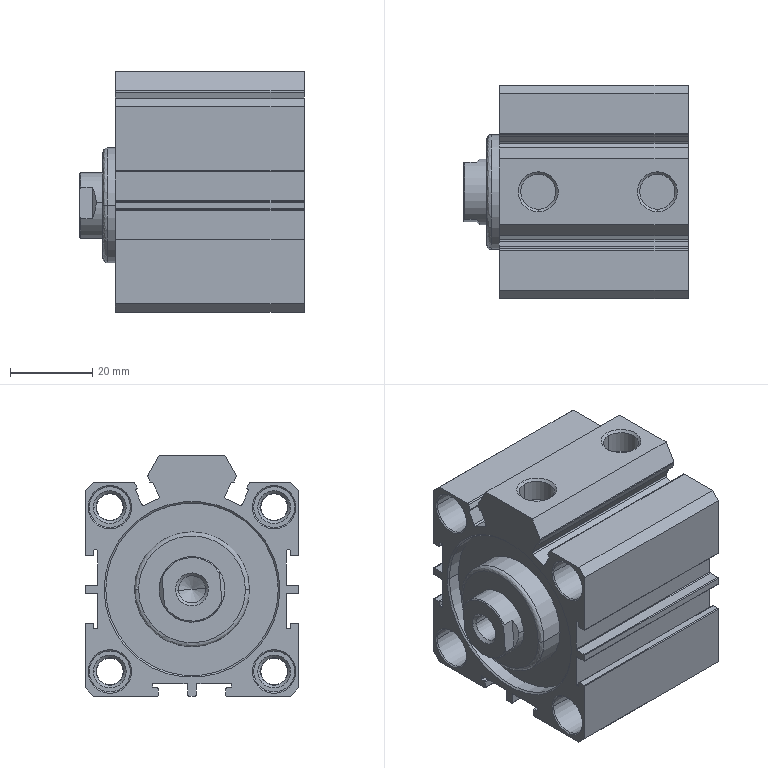Part | SolidWorks | 2 solids | 274 faces | box 54.62 x 52 x 58.5 mm | volume 87613 mm3 | cylinder 116 | plane 94 | cone 62 | spline 2 | commonest cylinder face diameters 0.4 x46 6.647 x18 10 x16 0.8 x10 6.5 x8 8.566 x4